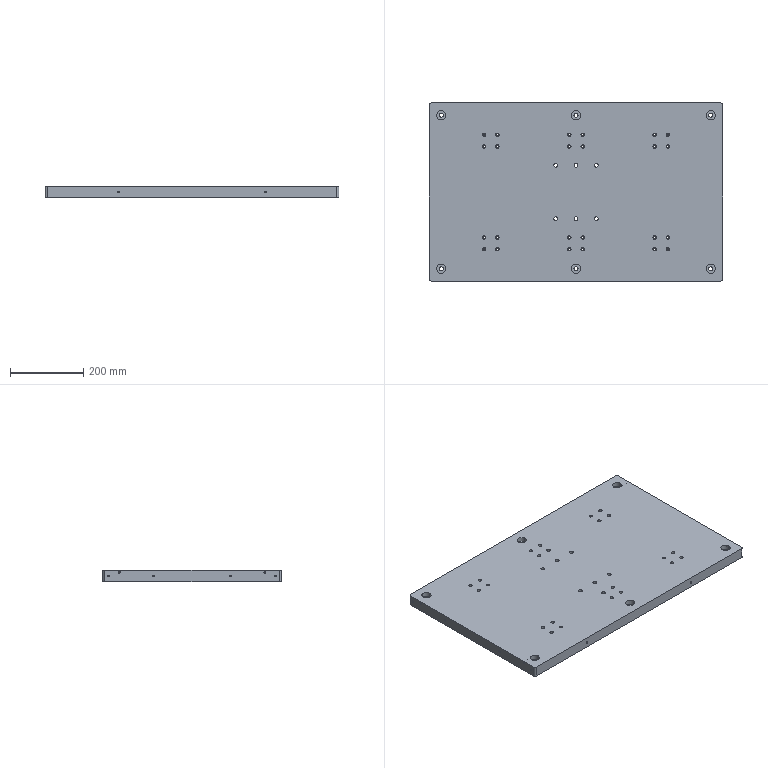NC program | Mastercam | posted with a generic post | part box 800 x 485 x 30 mm
Lines 4757 to 5950 of 7047:
N7890 T9 M6
N7900 G0 G90 G17 G54 X-361.57 Y208. A0. S6500 M3
N7910 G43 H9 Z50. M8
N7920 Z1.
N7930 G1 Z0. F600.
N7940 X-360.57 F3000.
N7950 G3 X-359.57 Y209. I0. J1.
N7960 X-367. Y216.43 Z-.175 I-7.43 J0.
N7970 X-374.43 Y209. Z-.35 I0. J-7.43
N7980 X-367. Y201.57 Z-.525 I7.43 J0.
N7990 X-359.57 Y209. Z-.7 I0. J7.43
N8000 X-367. Y216.43 Z-.875 I-7.43 J0.
N8010 X-374.43 Y209. Z-1.05 I0. J-7.43
N8020 X-367. Y201.57 Z-1.225 I7.43 J0.
N8030 X-359.57 Y209. Z-1.4 I0. J7.43
N8040 X-367. Y216.43 Z-1.575 I-7.43 J0.
N8050 X-374.43 Y209. Z-1.75 I0. J-7.43
N8060 X-367. Y201.57 Z-1.925 I7.43 J0.
N8070 X-359.57 Y209. Z-2.1 I0. J7.43
N8080 X-367. Y216.43 Z-2.275 I-7.43 J0.
N8090 X-374.43 Y209. Z-2.45 I0. J-7.43
N8100 X-367. Y201.57 Z-2.625 I7.43 J0.
N8110 X-359.57 Y209. Z-2.8 I0. J7.43
N8120 X-367. Y216.43 Z-2.975 I-7.43 J0.
N8130 X-374.43 Y209. Z-3.15 I0. J-7.43
N8140 X-367. Y201.57 Z-3.325 I7.43 J0.
N8150 X-359.57 Y209. Z-3.5 I0. J7.43
N8160 X-367. Y216.43 Z-3.675 I-7.43 J0.
N8170 X-374.43 Y209. Z-3.85 I0. J-7.43
N8180 X-367. Y201.57 Z-4.025 I7.43 J0.
N8190 X-359.57 Y209. Z-4.2 I0. J7.43
N8200 X-367. Y216.43 Z-4.375 I-7.43 J0.
N8210 X-374.43 Y209. Z-4.55 I0. J-7.43
N8220 X-367. Y201.57 Z-4.725 I7.43 J0.
N8230 X-359.57 Y209. Z-4.9 I0. J7.43
N8240 X-367. Y216.43 Z-5.075 I-7.43 J0.
N8250 X-374.43 Y209. Z-5.25 I0. J-7.43
N8260 X-367. Y201.57 Z-5.425 I7.43 J0.
N8270 X-359.57 Y209. Z-5.6 I0. J7.43
N8280 X-367. Y216.43 Z-5.775 I-7.43 J0.
N8290 X-374.43 Y209. Z-5.95 I0. J-7.43
N8300 X-367. Y201.57 Z-6.125 I7.43 J0.
N8310 X-359.57 Y209. Z-6.3 I0. J7.43
N8320 X-367. Y216.43 Z-6.475 I-7.43 J0.
N8330 X-374.43 Y209. Z-6.65 I0. J-7.43
N8340 X-367. Y201.57 Z-6.825 I7.43 J0.
N8350 X-359.57 Y209. Z-7. I0. J7.43
N8360 X-367. Y216.43 Z-7.175 I-7.43 J0.
N8370 X-374.43 Y209. Z-7.35 I0. J-7.43
N8380 X-367. Y201.57 Z-7.525 I7.43 J0.
N8390 X-359.57 Y209. Z-7.7 I0. J7.43
N8400 X-367. Y216.43 Z-7.875 I-7.43 J0.
N8410 X-374.43 Y209. Z-8.05 I0. J-7.43
N8420 X-367. Y201.57 Z-8.225 I7.43 J0.
N8430 X-359.57 Y209. Z-8.4 I0. J7.43
N8440 X-367. Y216.43 Z-8.575 I-7.43 J0.
N8450 X-374.43 Y209. Z-8.75 I0. J-7.43
N8460 X-367. Y201.57 Z-8.925 I7.43 J0.
N8470 X-359.57 Y209. Z-9.1 I0. J7.43
N8480 X-367. Y216.43 Z-9.275 I-7.43 J0.
N8490 X-374.43 Y209. Z-9.45 I0. J-7.43
N8500 X-367. Y201.57 Z-9.625 I7.43 J0.
N8510 X-359.57 Y209. Z-9.8 I0. J7.43
N8520 X-367. Y216.43 Z-9.975 I-7.43 J0.
N8530 X-374.43 Y209. Z-10.15 I0. J-7.43
N8540 X-367. Y201.57 Z-10.325 I7.43 J0.
N8550 X-359.57 Y209. Z-10.5 I0. J7.43
N8560 X-367. Y216.43 Z-10.675 I-7.43 J0.
N8570 X-374.43 Y209. Z-10.85 I0. J-7.43
N8580 X-367. Y201.57 Z-11.025 I7.43 J0.
N8590 X-359.57 Y209. Z-11.2 I0. J7.43
N8600 X-367. Y216.43 Z-11.375 I-7.43 J0.
N8610 X-374.43 Y209. Z-11.55 I0. J-7.43
N8620 X-367. Y201.57 Z-11.725 I7.43 J0.
N8630 X-359.57 Y209. Z-11.9 I0. J7.43
N8640 X-367. Y216.43 Z-12.075 I-7.43 J0.
N8650 X-374.43 Y209. Z-12.25 I0. J-7.43
N8660 X-367. Y201.57 Z-12.425 I7.43 J0.
N8670 X-359.57 Y209. Z-12.6 I0. J7.43
N8680 X-367. Y216.43 Z-12.775 I-7.43 J0.
N8690 X-373.694 Y212.224 Z-12.9 I0. J-7.43
N8700 X-374.43 Y209. I6.694 J-3.224
N8710 X-367. Y201.57 I7.43 J0.
N8720 X-359.57 Y209. I0. J7.43
N8730 X-367. Y216.43 I-7.43 J0.
N8740 X-373.694 Y212.224 I0. J-7.43
N8750 X-373.793 Y211.79 I.901 J-.434
N8760 X-373.227 Y210.889 I1. J0.
N8770 G1 X-372.326 Y210.455
N8780 G0 Z50.
N8790 X-361.57 Y-210.
N8800 Z1.
N8810 G1 Z0. F600.
N8820 X-360.57 F3000.
N8830 G3 X-359.57 Y-209. I0. J1.
N8840 X-367. Y-201.57 Z-.175 I-7.43 J0.
N8850 X-374.43 Y-209. Z-.35 I0. J-7.43
N8860 X-367. Y-216.43 Z-.525 I7.43 J0.
N8870 X-359.57 Y-209. Z-.7 I0. J7.43
N8880 X-367. Y-201.57 Z-.875 I-7.43 J0.
N8890 X-374.43 Y-209. Z-1.05 I0. J-7.43
N8900 X-367. Y-216.43 Z-1.225 I7.43 J0.
N8910 X-359.57 Y-209. Z-1.4 I0. J7.43
N8920 X-367. Y-201.57 Z-1.575 I-7.43 J0.
N8930 X-374.43 Y-209. Z-1.75 I0. J-7.43
N8940 X-367. Y-216.43 Z-1.925 I7.43 J0.
N8950 X-359.57 Y-209. Z-2.1 I0. J7.43
N8960 X-367. Y-201.57 Z-2.275 I-7.43 J0.
N8970 X-374.43 Y-209. Z-2.45 I0. J-7.43
N8980 X-367. Y-216.43 Z-2.625 I7.43 J0.
N8990 X-359.57 Y-209. Z-2.8 I0. J7.43
N9000 X-367. Y-201.57 Z-2.975 I-7.43 J0.
N9010 X-374.43 Y-209. Z-3.15 I0. J-7.43
N9020 X-367. Y-216.43 Z-3.325 I7.43 J0.
N9030 X-359.57 Y-209. Z-3.5 I0. J7.43
N9040 X-367. Y-201.57 Z-3.675 I-7.43 J0.
N9050 X-374.43 Y-209. Z-3.85 I0. J-7.43
N9060 X-367. Y-216.43 Z-4.025 I7.43 J0.
N9070 X-359.57 Y-209. Z-4.2 I0. J7.43
N9080 X-367. Y-201.57 Z-4.375 I-7.43 J0.
N9090 X-374.43 Y-209. Z-4.55 I0. J-7.43
N9100 X-367. Y-216.43 Z-4.725 I7.43 J0.
N9110 X-359.57 Y-209. Z-4.9 I0. J7.43
N9120 X-367. Y-201.57 Z-5.075 I-7.43 J0.
N9130 X-374.43 Y-209. Z-5.25 I0. J-7.43
N9140 X-367. Y-216.43 Z-5.425 I7.43 J0.
N9150 X-359.57 Y-209. Z-5.6 I0. J7.43
N9160 X-367. Y-201.57 Z-5.775 I-7.43 J0.
N9170 X-374.43 Y-209. Z-5.95 I0. J-7.43
N9180 X-367. Y-216.43 Z-6.125 I7.43 J0.
N9190 X-359.57 Y-209. Z-6.3 I0. J7.43
N9200 X-367. Y-201.57 Z-6.475 I-7.43 J0.
N9210 X-374.43 Y-209. Z-6.65 I0. J-7.43
N9220 X-367. Y-216.43 Z-6.825 I7.43 J0.
N9230 X-359.57 Y-209. Z-7. I0. J7.43
N9240 X-367. Y-201.57 Z-7.175 I-7.43 J0.
N9250 X-374.43 Y-209. Z-7.35 I0. J-7.43
N9260 X-367. Y-216.43 Z-7.525 I7.43 J0.
N9270 X-359.57 Y-209. Z-7.7 I0. J7.43
N9280 X-367. Y-201.57 Z-7.875 I-7.43 J0.
N9290 X-374.43 Y-209. Z-8.05 I0. J-7.43
N9300 X-367. Y-216.43 Z-8.225 I7.43 J0.
N9310 X-359.57 Y-209. Z-8.4 I0. J7.43
N9320 X-367. Y-201.57 Z-8.575 I-7.43 J0.
N9330 X-374.43 Y-209. Z-8.75 I0. J-7.43
N9340 X-367. Y-216.43 Z-8.925 I7.43 J0.
N9350 X-359.57 Y-209. Z-9.1 I0. J7.43
N9360 X-367. Y-201.57 Z-9.275 I-7.43 J0.
N9370 X-374.43 Y-209. Z-9.45 I0. J-7.43
N9380 X-367. Y-216.43 Z-9.625 I7.43 J0.
N9390 X-359.57 Y-209. Z-9.8 I0. J7.43
N9400 X-367. Y-201.57 Z-9.975 I-7.43 J0.
N9410 X-374.43 Y-209. Z-10.15 I0. J-7.43
N9420 X-367. Y-216.43 Z-10.325 I7.43 J0.
N9430 X-359.57 Y-209. Z-10.5 I0. J7.43
N9440 X-367. Y-201.57 Z-10.675 I-7.43 J0.
N9450 X-374.43 Y-209. Z-10.85 I0. J-7.43
N9460 X-367. Y-216.43 Z-11.025 I7.43 J0.
N9470 X-359.57 Y-209. Z-11.2 I0. J7.43
N9480 X-367. Y-201.57 Z-11.375 I-7.43 J0.
N9490 X-374.43 Y-209. Z-11.55 I0. J-7.43
N9500 X-367. Y-216.43 Z-11.725 I7.43 J0.
N9510 X-359.57 Y-209. Z-11.9 I0. J7.43
N9520 X-367. Y-201.57 Z-12.075 I-7.43 J0.
N9530 X-374.43 Y-209. Z-12.25 I0. J-7.43
N9540 X-367. Y-216.43 Z-12.425 I7.43 J0.
N9550 X-359.57 Y-209. Z-12.6 I0. J7.43
N9560 X-367. Y-201.57 Z-12.775 I-7.43 J0.
N9570 X-373.694 Y-205.776 Z-12.9 I0. J-7.43
N9580 X-374.43 Y-209. I6.694 J-3.224
N9590 X-367. Y-216.43 I7.43 J0.
N9600 X-359.57 Y-209. I0. J7.43
N9610 X-367. Y-201.57 I-7.43 J0.
N9620 X-373.694 Y-205.776 I0. J-7.43
N9630 X-373.793 Y-206.21 I.901 J-.434
N9640 X-373.227 Y-207.111 I1. J0.
N9650 G1 X-372.326 Y-207.545
N9660 G0 Z50.
N9670 X5.43 Y-210.
N9680 Z1.
N9690 G1 Z0. F600.
N9700 X6.43 F3000.
N9710 G3 X7.43 Y-209. I0. J1.
N9720 X0. Y-201.57 Z-.175 I-7.43 J0.
N9730 X-7.43 Y-209. Z-.35 I0. J-7.43
N9740 X0. Y-216.43 Z-.525 I7.43 J0.
N9750 X7.43 Y-209. Z-.7 I0. J7.43
N9760 X0. Y-201.57 Z-.875 I-7.43 J0.
N9770 X-7.43 Y-209. Z-1.05 I0. J-7.43
N9780 X0. Y-216.43 Z-1.225 I7.43 J0.
N9790 X7.43 Y-209. Z-1.4 I0. J7.43
N9800 X0. Y-201.57 Z-1.575 I-7.43 J0.
N9810 X-7.43 Y-209. Z-1.75 I0. J-7.43
N9820 X0. Y-216.43 Z-1.925 I7.43 J0.
N9830 X7.43 Y-209. Z-2.1 I0. J7.43
N9840 X0. Y-201.57 Z-2.275 I-7.43 J0.
N9850 X-7.43 Y-209. Z-2.45 I0. J-7.43
N9860 X0. Y-216.43 Z-2.625 I7.43 J0.
N9870 X7.43 Y-209. Z-2.8 I0. J7.43
N9880 X0. Y-201.57 Z-2.975 I-7.43 J0.
N9890 X-7.43 Y-209. Z-3.15 I0. J-7.43
N9900 X0. Y-216.43 Z-3.325 I7.43 J0.
N9910 X7.43 Y-209. Z-3.5 I0. J7.43
N9920 X0. Y-201.57 Z-3.675 I-7.43 J0.
N9930 X-7.43 Y-209. Z-3.85 I0. J-7.43
N9940 X0. Y-216.43 Z-4.025 I7.43 J0.
N9950 X7.43 Y-209. Z-4.2 I0. J7.43
N9960 X0. Y-201.57 Z-4.375 I-7.43 J0.
N9970 X-7.43 Y-209. Z-4.55 I0. J-7.43
N9980 X0. Y-216.43 Z-4.725 I7.43 J0.
N9990 X7.43 Y-209. Z-4.9 I0. J7.43
N100 X0. Y-201.57 Z-5.075 I-7.43 J0.
N110 X-7.43 Y-209. Z-5.25 I0. J-7.43
N120 X0. Y-216.43 Z-5.425 I7.43 J0.
N130 X7.43 Y-209. Z-5.6 I0. J7.43
N140 X0. Y-201.57 Z-5.775 I-7.43 J0.
N150 X-7.43 Y-209. Z-5.95 I0. J-7.43
N160 X0. Y-216.43 Z-6.125 I7.43 J0.
N170 X7.43 Y-209. Z-6.3 I0. J7.43
N180 X0. Y-201.57 Z-6.475 I-7.43 J0.
N190 X-7.43 Y-209. Z-6.65 I0. J-7.43
N200 X0. Y-216.43 Z-6.825 I7.43 J0.
N210 X7.43 Y-209. Z-7. I0. J7.43
N220 X0. Y-201.57 Z-7.175 I-7.43 J0.
N230 X-7.43 Y-209. Z-7.35 I0. J-7.43
N240 X0. Y-216.43 Z-7.525 I7.43 J0.
N250 X7.43 Y-209. Z-7.7 I0. J7.43
N260 X0. Y-201.57 Z-7.875 I-7.43 J0.
N270 X-7.43 Y-209. Z-8.05 I0. J-7.43
N280 X0. Y-216.43 Z-8.225 I7.43 J0.
N290 X7.43 Y-209. Z-8.4 I0. J7.43
N300 X0. Y-201.57 Z-8.575 I-7.43 J0.
N310 X-7.43 Y-209. Z-8.75 I0. J-7.43
N320 X0. Y-216.43 Z-8.925 I7.43 J0.
N330 X7.43 Y-209. Z-9.1 I0. J7.43
N340 X0. Y-201.57 Z-9.275 I-7.43 J0.
N350 X-7.43 Y-209. Z-9.45 I0. J-7.43
N360 X0. Y-216.43 Z-9.625 I7.43 J0.
N370 X7.43 Y-209. Z-9.8 I0. J7.43
N380 X0. Y-201.57 Z-9.975 I-7.43 J0.
N390 X-7.43 Y-209. Z-10.15 I0. J-7.43
N400 X0. Y-216.43 Z-10.325 I7.43 J0.
N410 X7.43 Y-209. Z-10.5 I0. J7.43
N420 X0. Y-201.57 Z-10.675 I-7.43 J0.
N430 X-7.43 Y-209. Z-10.85 I0. J-7.43
N440 X0. Y-216.43 Z-11.025 I7.43 J0.
N450 X7.43 Y-209. Z-11.2 I0. J7.43
N460 X0. Y-201.57 Z-11.375 I-7.43 J0.
N470 X-7.43 Y-209. Z-11.55 I0. J-7.43
N480 X0. Y-216.43 Z-11.725 I7.43 J0.
N490 X7.43 Y-209. Z-11.9 I0. J7.43
N500 X0. Y-201.57 Z-12.075 I-7.43 J0.
N510 X-7.43 Y-209. Z-12.25 I0. J-7.43
N520 X0. Y-216.43 Z-12.425 I7.43 J0.
N530 X7.43 Y-209. Z-12.6 I0. J7.43
N540 X0. Y-201.57 Z-12.775 I-7.43 J0.
N550 X-6.694 Y-205.776 Z-12.9 I0. J-7.43
N560 X-7.43 Y-209. I6.694 J-3.224
N570 X0. Y-216.43 I7.43 J0.
N580 X7.43 Y-209. I0. J7.43
N590 X0. Y-201.57 I-7.43 J0.
N600 X-6.694 Y-205.776 I0. J-7.43
N610 X-6.793 Y-206.21 I.901 J-.434
N620 X-6.227 Y-207.111 I1. J0.
N630 G1 X-5.326 Y-207.545
N640 G0 Z50.
N650 X5.43 Y208.
N660 Z1.
N670 G1 Z0. F600.
N680 X6.43 F3000.
N690 G3 X7.43 Y209. I0. J1.
N700 X0. Y216.43 Z-.175 I-7.43 J0.
N710 X-7.43 Y209. Z-.35 I0. J-7.43
N720 X0. Y201.57 Z-.525 I7.43 J0.
N730 X7.43 Y209. Z-.7 I0. J7.43
N740 X0. Y216.43 Z-.875 I-7.43 J0.
N750 X-7.43 Y209. Z-1.05 I0. J-7.43
N760 X0. Y201.57 Z-1.225 I7.43 J0.
N770 X7.43 Y209. Z-1.4 I0. J7.43
N780 X0. Y216.43 Z-1.575 I-7.43 J0.
N790 X-7.43 Y209. Z-1.75 I0. J-7.43
N800 X0. Y201.57 Z-1.925 I7.43 J0.
N810 X7.43 Y209. Z-2.1 I0. J7.43
N820 X0. Y216.43 Z-2.275 I-7.43 J0.
N830 X-7.43 Y209. Z-2.45 I0. J-7.43
N840 X0. Y201.57 Z-2.625 I7.43 J0.
N850 X7.43 Y209. Z-2.8 I0. J7.43
N860 X0. Y216.43 Z-2.975 I-7.43 J0.
N870 X-7.43 Y209. Z-3.15 I0. J-7.43
N880 X0. Y201.57 Z-3.325 I7.43 J0.
N890 X7.43 Y209. Z-3.5 I0. J7.43
N900 X0. Y216.43 Z-3.675 I-7.43 J0.
N910 X-7.43 Y209. Z-3.85 I0. J-7.43
N920 X0. Y201.57 Z-4.025 I7.43 J0.
N930 X7.43 Y209. Z-4.2 I0. J7.43
N940 X0. Y216.43 Z-4.375 I-7.43 J0.
N950 X-7.43 Y209. Z-4.55 I0. J-7.43
N960 X0. Y201.57 Z-4.725 I7.43 J0.
N970 X7.43 Y209. Z-4.9 I0. J7.43
N980 X0. Y216.43 Z-5.075 I-7.43 J0.
N990 X-7.43 Y209. Z-5.25 I0. J-7.43
N1000 X0. Y201.57 Z-5.425 I7.43 J0.
N1010 X7.43 Y209. Z-5.6 I0. J7.43
N1020 X0. Y216.43 Z-5.775 I-7.43 J0.
N1030 X-7.43 Y209. Z-5.95 I0. J-7.43
N1040 X0. Y201.57 Z-6.125 I7.43 J0.
N1050 X7.43 Y209. Z-6.3 I0. J7.43
N1060 X0. Y216.43 Z-6.475 I-7.43 J0.
N1070 X-7.43 Y209. Z-6.65 I0. J-7.43
N1080 X0. Y201.57 Z-6.825 I7.43 J0.
N1090 X7.43 Y209. Z-7. I0. J7.43
N1100 X0. Y216.43 Z-7.175 I-7.43 J0.
N1110 X-7.43 Y209. Z-7.35 I0. J-7.43
N1120 X0. Y201.57 Z-7.525 I7.43 J0.
N1130 X7.43 Y209. Z-7.7 I0. J7.43
N1140 X0. Y216.43 Z-7.875 I-7.43 J0.
N1150 X-7.43 Y209. Z-8.05 I0. J-7.43
N1160 X0. Y201.57 Z-8.225 I7.43 J0.
N1170 X7.43 Y209. Z-8.4 I0. J7.43
N1180 X0. Y216.43 Z-8.575 I-7.43 J0.
N1190 X-7.43 Y209. Z-8.75 I0. J-7.43
N1200 X0. Y201.57 Z-8.925 I7.43 J0.
N1210 X7.43 Y209. Z-9.1 I0. J7.43
N1220 X0. Y216.43 Z-9.275 I-7.43 J0.
N1230 X-7.43 Y209. Z-9.45 I0. J-7.43
N1240 X0. Y201.57 Z-9.625 I7.43 J0.
N1250 X7.43 Y209. Z-9.8 I0. J7.43
N1260 X0. Y216.43 Z-9.975 I-7.43 J0.
N1270 X-7.43 Y209. Z-10.15 I0. J-7.43
N1280 X0. Y201.57 Z-10.325 I7.43 J0.
N1290 X7.43 Y209. Z-10.5 I0. J7.43
N1300 X0. Y216.43 Z-10.675 I-7.43 J0.
N1310 X-7.43 Y209. Z-10.85 I0. J-7.43
N1320 X0. Y201.57 Z-11.025 I7.43 J0.
N1330 X7.43 Y209. Z-11.2 I0. J7.43
N1340 X0. Y216.43 Z-11.375 I-7.43 J0.
N1350 X-7.43 Y209. Z-11.55 I0. J-7.43
N1360 X0. Y201.57 Z-11.725 I7.43 J0.
N1370 X7.43 Y209. Z-11.9 I0. J7.43
N1380 X0. Y216.43 Z-12.075 I-7.43 J0.
N1390 X-7.43 Y209. Z-12.25 I0. J-7.43
N1400 X0. Y201.57 Z-12.425 I7.43 J0.
N1410 X7.43 Y209. Z-12.6 I0. J7.43
N1420 X0. Y216.43 Z-12.775 I-7.43 J0.
N1430 X-6.694 Y212.224 Z-12.9 I0. J-7.43
N1440 X-7.43 Y209. I6.694 J-3.224
N1450 X0. Y201.57 I7.43 J0.
N1460 X7.43 Y209. I0. J7.43
N1470 X0. Y216.43 I-7.43 J0.
N1480 X-6.694 Y212.224 I0. J-7.43
N1490 X-6.793 Y211.79 I.901 J-.434
N1500 X-6.227 Y210.889 I1. J0.
N1510 G1 X-5.326 Y210.455
N1520 G0 Z50.
N1530 X372.43 Y208.
N1540 Z1.
N1550 G1 Z0. F600.
N1560 X373.43 F3000.
N1570 G3 X374.43 Y209. I0. J1.
N1580 X367. Y216.43 Z-.175 I-7.43 J0.
N1590 X359.57 Y209. Z-.35 I0. J-7.43
N1600 X367. Y201.57 Z-.525 I7.43 J0.
N1610 X374.43 Y209. Z-.7 I0. J7.43
N1620 X367. Y216.43 Z-.875 I-7.43 J0.
N1630 X359.57 Y209. Z-1.05 I0. J-7.43
N1640 X367. Y201.57 Z-1.225 I7.43 J0.
N1650 X374.43 Y209. Z-1.4 I0. J7.43
N1660 X367. Y216.43 Z-1.575 I-7.43 J0.
N1670 X359.57 Y209. Z-1.75 I0. J-7.43
N1680 X367. Y201.57 Z-1.925 I7.43 J0.
N1690 X374.43 Y209. Z-2.1 I0. J7.43
N1700 X367. Y216.43 Z-2.275 I-7.43 J0.
N1710 X359.57 Y209. Z-2.45 I0. J-7.43
N1720 X367. Y201.57 Z-2.625 I7.43 J0.
N1730 X374.43 Y209. Z-2.8 I0. J7.43
N1740 X367. Y216.43 Z-2.975 I-7.43 J0.
N1750 X359.57 Y209. Z-3.15 I0. J-7.43
N1760 X367. Y201.57 Z-3.325 I7.43 J0.
N1770 X374.43 Y209. Z-3.5 I0. J7.43
N1780 X367. Y216.43 Z-3.675 I-7.43 J0.
N1790 X359.57 Y209. Z-3.85 I0. J-7.43
N1800 X367. Y201.57 Z-4.025 I7.43 J0.
N1810 X374.43 Y209. Z-4.2 I0. J7.43
N1820 X367. Y216.43 Z-4.375 I-7.43 J0.
N1830 X359.57 Y209. Z-4.55 I0. J-7.43
N1840 X367. Y201.57 Z-4.725 I7.43 J0.
N1850 X374.43 Y209. Z-4.9 I0. J7.43
N1860 X367. Y216.43 Z-5.075 I-7.43 J0.
N1870 X359.57 Y209. Z-5.25 I0. J-7.43
N1880 X367. Y201.57 Z-5.425 I7.43 J0.
N1890 X374.43 Y209. Z-5.6 I0. J7.43
N1900 X367. Y216.43 Z-5.775 I-7.43 J0.
N1910 X359.57 Y209. Z-5.95 I0. J-7.43
N1920 X367. Y201.57 Z-6.125 I7.43 J0.
N1930 X374.43 Y209. Z-6.3 I0. J7.43
N1940 X367. Y216.43 Z-6.475 I-7.43 J0.
N1950 X359.57 Y209. Z-6.65 I0. J-7.43
N1960 X367. Y201.57 Z-6.825 I7.43 J0.
N1970 X374.43 Y209. Z-7. I0. J7.43
N1980 X367. Y216.43 Z-7.175 I-7.43 J0.
N1990 X359.57 Y209. Z-7.35 I0. J-7.43
N2000 X367. Y201.57 Z-7.525 I7.43 J0.
N2010 X374.43 Y209. Z-7.7 I0. J7.43
N2020 X367. Y216.43 Z-7.875 I-7.43 J0.
N2030 X359.57 Y209. Z-8.05 I0. J-7.43
N2040 X367. Y201.57 Z-8.225 I7.43 J0.
N2050 X374.43 Y209. Z-8.4 I0. J7.43
N2060 X367. Y216.43 Z-8.575 I-7.43 J0.
N2070 X359.57 Y209. Z-8.75 I0. J-7.43
N2080 X367. Y201.57 Z-8.925 I7.43 J0.
N2090 X374.43 Y209. Z-9.1 I0. J7.43
N2100 X367. Y216.43 Z-9.275 I-7.43 J0.
N2110 X359.57 Y209. Z-9.45 I0. J-7.43
N2120 X367. Y201.57 Z-9.625 I7.43 J0.
N2130 X374.43 Y209. Z-9.8 I0. J7.43
N2140 X367. Y216.43 Z-9.975 I-7.43 J0.
N2150 X359.57 Y209. Z-10.15 I0. J-7.43
N2160 X367. Y201.57 Z-10.325 I7.43 J0.
N2170 X374.43 Y209. Z-10.5 I0. J7.43
N2180 X367. Y216.43 Z-10.675 I-7.43 J0.
N2190 X359.57 Y209. Z-10.85 I0. J-7.43
N2200 X367. Y201.57 Z-11.025 I7.43 J0.
N2210 X374.43 Y209. Z-11.2 I0. J7.43
N2220 X367. Y216.43 Z-11.375 I-7.43 J0.
N2230 X359.57 Y209. Z-11.55 I0. J-7.43
N2240 X367. Y201.57 Z-11.725 I7.43 J0.
N2250 X374.43 Y209. Z-11.9 I0. J7.43
N2260 X367. Y216.43 Z-12.075 I-7.43 J0.
N2270 X359.57 Y209. Z-12.25 I0. J-7.43
N2280 X367. Y201.57 Z-12.425 I7.43 J0.
N2290 X374.43 Y209. Z-12.6 I0. J7.43
N2300 X367. Y216.43 Z-12.775 I-7.43 J0.
N2310 X360.306 Y212.224 Z-12.9 I0. J-7.43
N2320 X359.57 Y209. I6.694 J-3.224
N2330 X367. Y201.57 I7.43 J0.
N2340 X374.43 Y209. I0. J7.43
N2350 X367. Y216.43 I-7.43 J0.
N2360 X360.306 Y212.224 I0. J-7.43
N2370 X360.207 Y211.79 I.901 J-.434
N2380 X360.773 Y210.889 I1. J0.
N2390 G1 X361.674 Y210.455
N2400 G0 Z50.
N2410 X372.43 Y-210.
N2420 Z1.
N2430 G1 Z0. F600.
N2440 X373.43 F3000.
N2450 G3 X374.43 Y-209. I0. J1.
N2460 X367. Y-201.57 Z-.175 I-7.43 J0.
N2470 X359.57 Y-209. Z-.35 I0. J-7.43
N2480 X367. Y-216.43 Z-.525 I7.43 J0.
N2490 X374.43 Y-209. Z-.7 I0. J7.43
N2500 X367. Y-201.57 Z-.875 I-7.43 J0.
N2510 X359.57 Y-209. Z-1.05 I0. J-7.43
N2520 X367. Y-216.43 Z-1.225 I7.43 J0.
N2530 X374.43 Y-209. Z-1.4 I0. J7.43
N2540 X367. Y-201.57 Z-1.575 I-7.43 J0.
N2550 X359.57 Y-209. Z-1.75 I0. J-7.43
N2560 X367. Y-216.43 Z-1.925 I7.43 J0.
N2570 X374.43 Y-209. Z-2.1 I0. J7.43
N2580 X367. Y-201.57 Z-2.275 I-7.43 J0.
N2590 X359.57 Y-209. Z-2.45 I0. J-7.43
N2600 X367. Y-216.43 Z-2.625 I7.43 J0.
N2610 X374.43 Y-209. Z-2.8 I0. J7.43
N2620 X367. Y-201.57 Z-2.975 I-7.43 J0.
N2630 X359.57 Y-209. Z-3.15 I0. J-7.43
N2640 X367. Y-216.43 Z-3.325 I7.43 J0.
N2650 X374.43 Y-209. Z-3.5 I0. J7.43
N2660 X367. Y-201.57 Z-3.675 I-7.43 J0.
N2670 X359.57 Y-209. Z-3.85 I0. J-7.43
N2680 X367. Y-216.43 Z-4.025 I7.43 J0.
N2690 X374.43 Y-209. Z-4.2 I0. J7.43
N2700 X367. Y-201.57 Z-4.375 I-7.43 J0.
N2710 X359.57 Y-209. Z-4.55 I0. J-7.43
N2720 X367. Y-216.43 Z-4.725 I7.43 J0.
N2730 X374.43 Y-209. Z-4.9 I0. J7.43
N2740 X367. Y-201.57 Z-5.075 I-7.43 J0.
N2750 X359.57 Y-209. Z-5.25 I0. J-7.43
N2760 X367. Y-216.43 Z-5.425 I7.43 J0.
N2770 X374.43 Y-209. Z-5.6 I0. J7.43
N2780 X367. Y-201.57 Z-5.775 I-7.43 J0.
N2790 X359.57 Y-209. Z-5.95 I0. J-7.43
N2800 X367. Y-216.43 Z-6.125 I7.43 J0.
N2810 X374.43 Y-209. Z-6.3 I0. J7.43
N2820 X367. Y-201.57 Z-6.475 I-7.43 J0.
N2830 X359.57 Y-209. Z-6.65 I0. J-7.43
N2840 X367. Y-216.43 Z-6.825 I7.43 J0.
N2850 X374.43 Y-209. Z-7. I0. J7.43
N2860 X367. Y-201.57 Z-7.175 I-7.43 J0.
N2870 X359.57 Y-209. Z-7.35 I0. J-7.43
N2880 X367. Y-216.43 Z-7.525 I7.43 J0.
N2890 X374.43 Y-209. Z-7.7 I0. J7.43
N2900 X367. Y-201.57 Z-7.875 I-7.43 J0.
N2910 X359.57 Y-209. Z-8.05 I0. J-7.43
N2920 X367. Y-216.43 Z-8.225 I7.43 J0.
N2930 X374.43 Y-209. Z-8.4 I0. J7.43
N2940 X367. Y-201.57 Z-8.575 I-7.43 J0.
N2950 X359.57 Y-209. Z-8.75 I0. J-7.43
N2960 X367. Y-216.43 Z-8.925 I7.43 J0.
N2970 X374.43 Y-209. Z-9.1 I0. J7.43
N2980 X367. Y-201.57 Z-9.275 I-7.43 J0.
N2990 X359.57 Y-209. Z-9.45 I0. J-7.43
N3000 X367. Y-216.43 Z-9.625 I7.43 J0.
N3010 X374.43 Y-209. Z-9.8 I0. J7.43
N3020 X367. Y-201.57 Z-9.975 I-7.43 J0.
N3030 X359.57 Y-209. Z-10.15 I0. J-7.43
N3040 X367. Y-216.43 Z-10.325 I7.43 J0.
N3050 X374.43 Y-209. Z-10.5 I0. J7.43
N3060 X367. Y-201.57 Z-10.675 I-7.43 J0.
N3070 X359.57 Y-209. Z-10.85 I0. J-7.43
N3080 X367. Y-216.43 Z-11.025 I7.43 J0.
N3090 X374.43 Y-209. Z-11.2 I0. J7.43
N3100 X367. Y-201.57 Z-11.375 I-7.43 J0.
N3110 X359.57 Y-209. Z-11.55 I0. J-7.43
N3120 X367. Y-216.43 Z-11.725 I7.43 J0.
N3130 X374.43 Y-209. Z-11.9 I0. J7.43
N3140 X367. Y-201.57 Z-12.075 I-7.43 J0.
N3150 X359.57 Y-209. Z-12.25 I0. J-7.43
N3160 X367. Y-216.43 Z-12.425 I7.43 J0.
N3170 X374.43 Y-209. Z-12.6 I0. J7.43
N3180 X367. Y-201.57 Z-12.775 I-7.43 J0.
N3190 X360.306 Y-205.776 Z-12.9 I0. J-7.43
N3200 X359.57 Y-209. I6.694 J-3.224
N3210 X367. Y-216.43 I7.43 J0.
N3220 X374.43 Y-209. I0. J7.43
N3230 X367. Y-201.57 I-7.43 J0.
N3240 X360.306 Y-205.776 I0. J-7.43
N3250 X360.207 Y-206.21 I.901 J-.434
N3260 X360.773 Y-207.111 I1. J0.
N3270 G1 X361.674 Y-207.545
N3280 G0 Z50.
N3290 M5
N3300 G91 G28 Z0. M9
N3310 A0.
N3320 M01
N3330 T10 M6
N3340 G0 G90 G17 G54 X-361.48 Y208. A0. S6500 M3
N3350 G43 H10 Z50. M8
N3360 Z1.
N3370 G1 Z-13. F600.
N3380 G41 D10 X-360.48 F1000.
N3390 G3 X-359.48 Y209. I0. J1.
N3400 X-367. Y216.52 I-7.52 J0.
N3410 X-374.52 Y209. I0. J-7.52
N3420 X-367. Y201.48 I7.52 J0.
N3430 X-359.48 Y209. I0. J7.52
N3440 X-360.48 Y210. I-1. J0.
N3450 G1 G40 X-361.48
N3460 G0 Z50.
N3470 Y208.
N3480 Z1.
N3490 G1 Z-13. F600.
N3500 G41 D10 X-360.48 F1000.
N3510 G3 X-359.48 Y209. I0. J1.
N3520 X-367. Y216.52 I-7.52 J0.
N3530 X-374.52 Y209. I0. J-7.52
N3540 X-367. Y201.48 I7.52 J0.
N3550 X-359.48 Y209. I0. J7.52
N3560 X-360.48 Y210. I-1. J0.
N3570 G1 G40 X-361.48
N3580 G0 Z50.
N3590 Y-210.
N3600 Z1.
N3610 G1 Z-13. F600.
N3620 G41 D10 X-360.48 F1000.
N3630 G3 X-359.48 Y-209. I0. J1.
N3640 X-367. Y-201.48 I-7.52 J0.
N3650 X-374.52 Y-209. I0. J-7.52
N3660 X-367. Y-216.52 I7.52 J0.
N3670 X-359.48 Y-209. I0. J7.52
N3680 X-360.48 Y-208. I-1. J0.
N3690 G1 G40 X-361.48
N3700 G0 Z50.
N3710 Y-210.
N3720 Z1.
N3730 G1 Z-13. F600.
N3740 G41 D10 X-360.48 F1000.
N3750 G3 X-359.48 Y-209. I0. J1.
N3760 X-367. Y-201.48 I-7.52 J0.
N3770 X-374.52 Y-209. I0. J-7.52
N3780 X-367. Y-216.52 I7.52 J0.
N3790 X-359.48 Y-209. I0. J7.52
N3800 X-360.48 Y-208. I-1. J0.
N3810 G1 G40 X-361.48
N3820 G0 Z50.
N3830 X5.52 Y-210.
N3840 Z1.
N3850 G1 Z-13. F600.
N3860 G41 D10 X6.52 F1000.
N3870 G3 X7.52 Y-209. I0. J1.
N3880 X0. Y-201.48 I-7.52 J0.
N3890 X-7.52 Y-209. I0. J-7.52
N3900 X0. Y-216.52 I7.52 J0.
N3910 X7.52 Y-209. I0. J7.52
N3920 X6.52 Y-208. I-1. J0.
N3930 G1 G40 X5.52
N3940 G0 Z50.
N3950 Y-210.
N3960 Z1.
N3970 G1 Z-13. F600.
N3980 G41 D10 X6.52 F1000.
N3990 G3 X7.52 Y-209. I0. J1.
N4000 X0. Y-201.48 I-7.52 J0.
N4010 X-7.52 Y-209. I0. J-7.52
N4020 X0. Y-216.52 I7.52 J0.
N4030 X7.52 Y-209. I0. J7.52
N4040 X6.52 Y-208. I-1. J0.
N4050 G1 G40 X5.52
N4060 G0 Z50.
N4070 Y208.
N4080 Z1.
N4090 G1 Z-13. F600.
N4100 G41 D10 X6.52 F1000.
N4110 G3 X7.52 Y209. I0. J1.
N4120 X0. Y216.52 I-7.52 J0.
N4130 X-7.52 Y209. I0. J-7.52
N4140 X0. Y201.48 I7.52 J0.
N4150 X7.52 Y209. I0. J7.52
N4160 X6.52 Y210. I-1. J0.
N4170 G1 G40 X5.52
N4180 G0 Z50.
N4190 Y208.
N4200 Z1.
N4210 G1 Z-13. F600.
N4220 G41 D10 X6.52 F1000.
N4230 G3 X7.52 Y209. I0. J1.
N4240 X0. Y216.52 I-7.52 J0.
N4250 X-7.52 Y209. I0. J-7.52
N4260 X0. Y201.48 I7.52 J0.
N4270 X7.52 Y209. I0. J7.52
N4280 X6.52 Y210. I-1. J0.
N4290 G1 G40 X5.52
N4300 G0 Z50.
N4310 X372.52 Y208.
N4320 Z1.
N4330 G1 Z-13. F600.
N4340 G41 D10 X373.52 F1000.
N4350 G3 X374.52 Y209. I0. J1.
N4360 X367. Y216.52 I-7.52 J0.
N4370 X359.48 Y209. I0. J-7.52
N4380 X367. Y201.48 I7.52 J0.
N4390 X374.52 Y209. I0. J7.52
N4400 X373.52 Y210. I-1. J0.
N4410 G1 G40 X372.52
N4420 G0 Z50.
N4430 Y208.
N4440 Z1.
N4450 G1 Z-13. F600.
N4460 G41 D10 X373.52 F1000.
N4470 G3 X374.52 Y209. I0. J1.
N4480 X367. Y216.52 I-7.52 J0.
N4490 X359.48 Y209. I0. J-7.52
N4500 X367. Y201.48 I7.52 J0.
N4510 X374.52 Y209. I0. J7.52
N4520 X373.52 Y210. I-1. J0.
N4530 G1 G40 X372.52
N4540 G0 Z50.
N4550 Y-210.
N4560 Z1.
N4570 G1 Z-13. F600.
N4580 G41 D10 X373.52 F1000.
N4590 G3 X374.52 Y-209. I0. J1.
N4600 X367. Y-201.48 I-7.52 J0.
N4610 X359.48 Y-209. I0. J-7.52
N4620 X367. Y-216.52 I7.52 J0.
N4630 X374.52 Y-209. I0. J7.52
N4640 X373.52 Y-208. I-1. J0.
N4650 G1 G40 X372.52
N4660 G0 Z50.
N4670 Y-210.
N4680 Z1.
N4690 G1 Z-13. F600.
N4700 G41 D10 X373.52 F1000.
N4710 G3 X374.52 Y-209. I0. J1.
N4720 X367. Y-201.48 I-7.52 J0.
N4730 X359.48 Y-209. I0. J-7.52
N4740 X367. Y-216.52 I7.52 J0.
N4750 X374.52 Y-209. I0. J7.52
N4760 X373.52 Y-208. I-1. J0.
N4770 G1 G40 X372.52
N4780 G0 Z50.
N4790 M5
N4800 G91 G28 Z0. M9
N4810 A0.
N4820 M01
N4830 T7 M6
N4840 G0 G90 G17 G54 X-51.2 Y-72.9 A0. S6000 M3
N4850 G43 H7 Z50. M8
N4860 Z1.
N4870 G1 Z-.8 F600.
N4880 X-50.8 F1000.
N4890 G3 X-50.4 Y-72.5 I0. J.4
N4900 X-55. Y-67.9 I-4.6 J0.
N4910 X-59.6 Y-72.5 I0. J-4.6
N4920 X-55. Y-77.1 I4.6 J0.
N4930 X-50.4 Y-72.5 I0. J4.6
N4940 X-50.8 Y-72.1 I-.4 J0.
N4950 G1 X-51.2
N4960 G0 Z50.
N4970 X3.8 Y-72.9
N4980 Z1.
N4990 G1 Z-.8 F600.
N5000 X4.2 F1000.
N5010 G3 X4.6 Y-72.5 I0. J.4
N5020 X0. Y-67.9 I-4.6 J0.
N5030 X-4.6 Y-72.5 I0. J-4.6
N5040 X0. Y-77.1 I4.6 J0.
N5050 X4.6 Y-72.5 I0. J4.6
N5060 X4.2 Y-72.1 I-.4 J0.
N5070 G1 X3.8
N5080 G0 Z50.
N5090 X58.8 Y-72.9
N5100 Z1.
N5110 G1 Z-.8 F600.
N5120 X59.2 F1000.
N5130 G3 X59.6 Y-72.5 I0. J.4
N5140 X55. Y-67.9 I-4.6 J0.
N5150 X50.4 Y-72.5 I0. J-4.6
N5160 X55. Y-77.1 I4.6 J0.
N5170 X59.6 Y-72.5 I0. J4.6
N5180 X59.2 Y-72.1 I-.4 J0.
N5190 G1 X58.8
N5200 G0 Z50.
N5210 X-51.2 Y72.1
N5220 Z1.
N5230 G1 Z-.8 F600.
N5240 X-50.8 F1000.
N5250 G3 X-50.4 Y72.5 I0. J.4
N5260 X-55. Y77.1 I-4.6 J0.
N5270 X-59.6 Y72.5 I0. J-4.6
N5280 X-55. Y67.9 I4.6 J0.
N5290 X-50.4 Y72.5 I0. J4.6
N5300 X-50.8 Y72.9 I-.4 J0.
N5310 G1 X-51.2
N5320 G0 Z50.
N5330 X3.8 Y72.1
N5340 Z1.
N5350 G1 Z-.8 F600.
N5360 X4.2 F1000.
N5370 G3 X4.6 Y72.5 I0. J.4
N5380 X0. Y77.1 I-4.6 J0.
N5390 X-4.6 Y72.5 I0. J-4.6
N5400 X0. Y67.9 I4.6 J0.
N5410 X4.6 Y72.5 I0. J4.6
N5420 X4.2 Y72.9 I-.4 J0.
N5430 G1 X3.8
N5440 G0 Z50.
N5450 X58.8 Y72.1
N5460 Z1.
N5470 G1 Z-.8 F600.
N5480 X59.2 F1000.
N5490 G3 X59.6 Y72.5 I0. J.4
N5500 X55. Y77.1 I-4.6 J0.
N5510 X50.4 Y72.5 I0. J-4.6
N5520 X55. Y67.9 I4.6 J0.
N5530 X59.6 Y72.5 I0. J4.6
N5540 X59.2 Y72.9 I-.4 J0.
N5550 G1 X58.8
N5560 G0 Z50.
N5570 X217.05 Y-124.4
N5580 Z1.
N5590 G1 Z-.8 F600.
N5600 X217.45 F1000.
N5610 G3 X217.85 Y-124. I0. J.4
N5620 X214. Y-120.15 I-3.85 J0.
N5630 X210.15 Y-124. I0. J-3.85
N5640 X214. Y-127.85 I3.85 J0.
N5650 X217.85 Y-124. I0. J3.85
N5660 X217.45 Y-123.6 I-.4 J0.
N5670 G1 X217.05
N5680 G0 Z50.
N5690 X253.05 Y155.6
N5700 Z1.
N5710 G1 Z-.8 F600.
N5720 X253.45 F1000.
N5730 G3 X253.85 Y156. I0. J.4
N5740 X250. Y159.85 I-3.85 J0.
N5750 X246.15 Y156. I0. J-3.85
N5760 X250. Y152.15 I3.85 J0.
N5770 X253.85 Y156. I0. J3.85
N5780 X253.45 Y156.4 I-.4 J0.
N5790 G1 X253.05
N5800 G0 Z50.
N5810 Y123.6
N5820 Z1.
N5830 G1 Z-.8 F600.
N5840 X253.45 F1000.
N5850 G3 X253.85 Y124. I0. J.4
N5860 X250. Y127.85 I-3.85 J0.
N5870 X246.15 Y124. I0. J-3.85
N5880 X250. Y120.15 I3.85 J0.
N5890 X253.85 Y124. I0. J3.85
N5900 X253.45 Y124.4 I-.4 J0.
N5910 G1 X253.05
N5920 G0 Z50.
N5930 X217.05 Y123.6
N5940 Z1.
N5950 G1 Z-.8 F600.
N5960 X217.45 F1000.
N5970 G3 X217.85 Y124. I0. J.4
N5980 X214. Y127.85 I-3.85 J0.
N5990 X210.15 Y124. I0. J-3.85
N6000 X214. Y120.15 I3.85 J0.
N6010 X217.85 Y124. I0. J3.85
N6020 X217.45 Y124.4 I-.4 J0.
N6030 G1 X217.05
N6040 G0 Z50.
N6050 Y-156.4
N6060 Z1.
N6070 G1 Z-.8 F600.
N6080 X217.45 F1000.
N6090 G3 X217.85 Y-156. I0. J.4
N6100 X214. Y-152.15 I-3.85 J0.
N6110 X210.15 Y-156. I0. J-3.85
N6120 X214. Y-159.85 I3.85 J0.
N6130 X217.85 Y-156. I0. J3.85
N6140 X217.45 Y-155.6 I-.4 J0.
N6150 G1 X217.05
N6160 G0 Z50.
N6170 X253.05 Y-156.4
N6180 Z1.
N6190 G1 Z-.8 F600.
N6200 X253.45 F1000.
N6210 G3 X253.85 Y-156. I0. J.4
N6220 X250. Y-152.15 I-3.85 J0.
N6230 X246.15 Y-156. I0. J-3.85
N6240 X250. Y-159.85 I3.85 J0.
N6250 X253.85 Y-156. I0. J3.85
N6260 X253.45 Y-155.6 I-.4 J0.
N6270 G1 X253.05
N6280 G0 Z50.
N6290 Y-124.4
N6300 Z1.
N6310 G1 Z-.8 F600.
N6320 X253.45 F1000.
N6330 G3 X253.85 Y-124. I0. J.4
N6340 X250. Y-120.15 I-3.85 J0.
N6350 X246.15 Y-124. I0. J-3.85
N6360 X250. Y-127.85 I3.85 J0.
N6370 X253.85 Y-124. I0. J3.85
N6380 X253.45 Y-123.6 I-.4 J0.
N6390 G1 X253.05
N6400 G0 Z50.
N6410 X21.05 Y-124.4
N6420 Z1.
N6430 G1 Z-.8 F600.
N6440 X21.45 F1000.
N6450 G3 X21.85 Y-124. I0. J.4
N6460 X18. Y-120.15 I-3.85 J0.
N6470 X14.15 Y-124. I0. J-3.85
N6480 X18. Y-127.85 I3.85 J0.
N6490 X21.85 Y-124. I0. J3.85
N6500 X21.45 Y-123.6 I-.4 J0.
N6510 G1 X21.05
N6520 G0 Z50.
N6530 X-246.95 Y123.6
N6540 Z1.
N6550 G1 Z-.8 F600.
N6560 X-246.55 F1000.
N6570 G3 X-246.15 Y124. I0. J.4
N6580 X-250. Y127.85 I-3.85 J0.
N6590 X-253.85 Y124. I0. J-3.85
N6600 X-250. Y120.15 I3.85 J0.
N6610 X-246.15 Y124. I0. J3.85
N6620 X-246.55 Y124.4 I-.4 J0.
N6630 G1 X-246.95
N6640 G0 Z50.
N6650 X-210.95 Y123.6
N6660 Z1.
N6670 G1 Z-.8 F600.
N6680 X-210.55 F1000.
N6690 G3 X-210.15 Y124. I0. J.4
N6700 X-214. Y127.85 I-3.85 J0.
N6710 X-217.85 Y124. I0. J-3.85
N6720 X-214. Y120.15 I3.85 J0.
N6730 X-210.15 Y124. I0. J3.85
N6740 X-210.55 Y124.4 I-.4 J0.
N6750 G1 X-210.95
N6760 G0 Z50.
N6770 Y155.6
N6780 Z1.
N6790 G1 Z-.8 F600.
N6800 X-210.55 F1000.
N6810 G3 X-210.15 Y156. I0. J.4
N6820 X-214. Y159.85 I-3.85 J0.
N6830 X-217.85 Y156. I0. J-3.85
N6840 X-214. Y152.15 I3.85 J0.
N6850 X-210.15 Y156. I0. J3.85
N6860 X-210.55 Y156.4 I-.4 J0.
N6870 G1 X-210.95
N6880 G0 Z50.
N6890 X-14.95 Y155.6
N6900 Z1.
N6910 G1 Z-.8 F600.
N6920 X-14.55 F1000.
N6930 G3 X-14.15 Y156. I0. J.4
N6940 X-18. Y159.85 I-3.85 J0.
N6950 X-21.85 Y156. I0. J-3.85
N6960 X-18. Y152.15 I3.85 J0.
N6970 X-14.15 Y156. I0. J3.85
N6980 X-14.55 Y156.4 I-.4 J0.
N6990 G1 X-14.95
N7000 G0 Z50.
N7010 Y123.6
N7020 Z1.
N7030 G1 Z-.8 F600.
N7040 X-14.55 F1000.
N7050 G3 X-14.15 Y124. I0. J.4
N7060 X-18. Y127.85 I-3.85 J0.
N7070 X-21.85 Y124. I0. J-3.85
N7080 X-18. Y120.15 I3.85 J0.
N7090 X-14.15 Y124. I0. J3.85
N7100 X-14.55 Y124.4 I-.4 J0.
N7110 G1 X-14.95
N7120 G0 Z50.
N7130 X21.05 Y123.6
N7140 Z1.
N7150 G1 Z-.8 F600.
N7160 X21.45 F1000.
N7170 G3 X21.85 Y124. I0. J.4
N7180 X18. Y127.85 I-3.85 J0.
N7190 X14.15 Y124. I0. J-3.85
N7200 X18. Y120.15 I3.85 J0.
N7210 X21.85 Y124. I0. J3.85
N7220 X21.45 Y124.4 I-.4 J0.
N7230 G1 X21.05
N7240 G0 Z50.
N7250 Y155.6
N7260 Z1.
N7270 G1 Z-.8 F600.
N7280 X21.45 F1000.
N7290 G3 X21.85 Y156. I0. J.4
N7300 X18. Y159.85 I-3.85 J0.
N7310 X14.15 Y156. I0. J-3.85
N7320 X18. Y152.15 I3.85 J0.
N7330 X21.85 Y156. I0. J3.85
N7340 X21.45 Y156.4 I-.4 J0.
N7350 G1 X21.05
N7360 G0 Z50.
N7370 X217.05 Y155.6
N7380 Z1.
N7390 G1 Z-.8 F600.
N7400 X217.45 F1000.
N7410 G3 X217.85 Y156. I0. J.4
N7420 X214. Y159.85 I-3.85 J0.
N7430 X210.15 Y156. I0. J-3.85
N7440 X214. Y152.15 I3.85 J0.
N7450 X217.85 Y156. I0. J3.85
N7460 X217.45 Y156.4 I-.4 J0.
N7470 G1 X217.05
N7480 G0 Z50.
N7490 X-210.95 Y-124.4
N7500 Z1.
N7510 G1 Z-.8 F600.
N7520 X-210.55 F1000.
N7530 G3 X-210.15 Y-124. I0. J.4
N7540 X-214. Y-120.15 I-3.85 J0.
N7550 X-217.85 Y-124. I0. J-3.85
N7560 X-214. Y-127.85 I3.85 J0.
N7570 X-210.15 Y-124. I0. J3.85
N7580 X-210.55 Y-123.6 I-.4 J0.
N7590 G1 X-210.95
N7600 G0 Z50.
N7610 Y-156.4
N7620 Z1.
N7630 G1 Z-.8 F600.
N7640 X-210.55 F1000.
N7650 G3 X-210.15 Y-156. I0. J.4
N7660 X-214. Y-152.15 I-3.85 J0.
N7670 X-217.85 Y-156. I0. J-3.85
N7680 X-214. Y-159.85 I3.85 J0.
N7690 X-210.15 Y-156. I0. J3.85
N7700 X-210.55 Y-155.6 I-.4 J0.
N7710 G1 X-210.95
N7720 G0 Z50.
N7730 X-246.95 Y-156.4
N7740 Z1.
N7750 G1 Z-.8 F600.
N7760 X-246.55 F1000.
N7770 G3 X-246.15 Y-156. I0. J.4
N7780 X-250. Y-152.15 I-3.85 J0.
N7790 X-253.85 Y-156. I0. J-3.85
N7800 X-250. Y-159.85 I3.85 J0.
N7810 X-246.15 Y-156. I0. J3.85
N7820 X-246.55 Y-155.6 I-.4 J0.
N7830 G1 X-246.95
N7840 G0 Z50.
N7850 Y-124.4
N7860 Z1.
N7870 G1 Z-.8 F600.
N7880 X-246.55 F1000.
N7890 G3 X-246.15 Y-124. I0. J.4
N7900 X-250. Y-120.15 I-3.85 J0.
N7910 X-253.85 Y-124. I0. J-3.85
N7920 X-250. Y-127.85 I3.85 J0.
N7930 X-246.15 Y-124. I0. J3.85
N7940 X-246.55 Y-123.6 I-.4 J0.
N7950 G1 X-246.95
N7960 G0 Z50.
N7970 X-14.95 Y-124.4
N7980 Z1.
N7990 G1 Z-.8 F600.
N8000 X-14.55 F1000.
N8010 G3 X-14.15 Y-124. I0. J.4
N8020 X-18. Y-120.15 I-3.85 J0.
N8030 X-21.85 Y-124. I0. J-3.85
N8040 X-18. Y-127.85 I3.85 J0.
N8050 X-14.15 Y-124. I0. J3.85
N8060 X-14.55 Y-123.6 I-.4 J0.
N8070 G1 X-14.95
N8080 G0 Z50.
N8090 Y-156.4
N8100 Z1.
N8110 G1 Z-.8 F600.
N8120 X-14.55 F1000.
N8130 G3 X-14.15 Y-156. I0. J.4
N8140 X-18. Y-152.15 I-3.85 J0.
N8150 X-21.85 Y-156. I0. J-3.85
N8160 X-18. Y-159.85 I3.85 J0.
N8170 X-14.15 Y-156. I0. J3.85
N8180 X-14.55 Y-155.6 I-.4 J0.
N8190 G1 X-14.95
N8200 G0 Z50.
N8210 X21.05 Y-156.4
N8220 Z1.
N8230 G1 Z-.8 F600.
N8240 X21.45 F1000.
N8250 G3 X21.85 Y-156. I0. J.4
N8260 X18. Y-152.15 I-3.85 J0.
N8270 X14.15 Y-156. I0. J-3.85
N8280 X18. Y-159.85 I3.85 J0.
N8290 X21.85 Y-156. I0. J3.85
N8300 X21.45 Y-155.6 I-.4 J0.
N8310 G1 X21.05
N8320 G0 Z50.
N8330 X-246.95 Y155.6
N8340 Z1.
N8350 G1 Z-.8 F600.
N8360 X-246.55 F1000.
N8370 G3 X-246.15 Y156. I0. J.4
N8380 X-250. Y159.85 I-3.85 J0.
N8390 X-253.85 Y156. I0. J-3.85
N8400 X-250. Y152.15 I3.85 J0.
N8410 X-246.15 Y156. I0. J3.85
N8420 X-246.55 Y156.4 I-.4 J0.
N8430 G1 X-246.95
N8440 G0 Z50.
N8450 X-355.95 Y-209.4
N8460 Z1.
N8470 G1 Z-.8 F600.
N8480 X-355.55 F1000.
N8490 G3 X-355.15 Y-209. I0. J.4
N8500 X-367. Y-197.15 I-11.85 J0.
N8510 X-378.85 Y-209. I0. J-11.85
N8520 X-367. Y-220.85 I11.85 J0.
N8530 X-355.15 Y-209. I0. J11.85
N8540 X-355.55 Y-208.6 I-.4 J0.
N8550 G1 X-355.95
N8560 G0 Z50.
N8570 X11.05 Y-209.4
N8580 Z1.
N8590 G1 Z-.8 F600.
N8600 X11.45 F1000.
N8610 G3 X11.85 Y-209. I0. J.4
N8620 X0. Y-197.15 I-11.85 J0.
N8630 X-11.85 Y-209. I0. J-11.85
N8640 X0. Y-220.85 I11.85 J0.
N8650 X11.85 Y-209. I0. J11.85
N8660 X11.45 Y-208.6 I-.4 J0.
N8670 G1 X11.05
N8680 G0 Z50.
N8690 X378.05 Y-209.4
N8700 Z1.
N8710 G1 Z-.8 F600.
N8720 X378.45 F1000.
N8730 G3 X378.85 Y-209. I0. J.4
N8740 X367. Y-197.15 I-11.85 J0.
N8750 X355.15 Y-209. I0. J-11.85
N8760 X367. Y-220.85 I11.85 J0.
N8770 X378.85 Y-209. I0. J11.85
N8780 X378.45 Y-208.6 I-.4 J0.
N8790 G1 X378.05
N8800 G0 Z50.
N8810 Y208.6
N8820 Z1.
N8830 G1 Z-.8 F600.
N8840 X378.45 F1000.
N8850 G3 X378.85 Y209. I0. J.4
N8860 X367. Y220.85 I-11.85 J0.
N8870 X355.15 Y209. I0. J-11.85
N8880 X367. Y197.15 I11.85 J0.
N8890 X378.85 Y209. I0. J11.85
N8900 X378.45 Y209.4 I-.4 J0.
N8910 G1 X378.05
N8920 G0 Z50.
N8930 X11.05 Y208.6
N8940 Z1.
N8950 G1 Z-.8 F600.
N8960 X11.45 F1000.
N8970 G3 X11.85 Y209. I0. J.4
N8980 X0. Y220.85 I-11.85 J0.
N8990 X-11.85 Y209. I0. J-11.85
N9000 X0. Y197.15 I11.85 J0.
N9010 X11.85 Y209. I0. J11.85
N9020 X11.45 Y209.4 I-.4 J0.
N9030 G1 X11.05
N9040 G0 Z50.
N9050 X-355.95 Y208.6
N9060 Z1.
N9070 G1 Z-.8 F600.
N9080 X-355.55 F1000.
N9090 G3 X-355.15 Y209. I0. J.4
N9100 X-367. Y220.85 I-11.85 J0.
N9110 X-378.85 Y209. I0. J-11.85
N9120 X-367. Y197.15 I11.85 J0.
N9130 X-355.15 Y209. I0. J11.85
N9140 X-355.55 Y209.4 I-.4 J0.
N9150 G1 X-355.95
N9160 G0 Z50.
N9170 X-362.95 Y-209.4
N9180 Z-12.
N9190 G1 Z-13.8 F600.
N9200 X-362.55 F1000.
N9210 G3 X-362.15 Y-209. I0. J.4
N9220 X-367. Y-204.15 I-4.85 J0.
N9230 X-371.85 Y-209. I0. J-4.85
N9240 X-367. Y-213.85 I4.85 J0.
N9250 X-362.15 Y-209. I0. J4.85
N9260 X-362.55 Y-208.6 I-.4 J0.
N9270 G1 X-362.95
N9280 G0 Z50.
N9290 X4.05 Y-209.4
N9300 Z-12.
N9310 G1 Z-13.8 F600.
N9320 X4.45 F1000.
N9330 G3 X4.85 Y-209. I0. J.4
N9340 X0. Y-204.15 I-4.85 J0.
N9350 X-4.85 Y-209. I0. J-4.85
N9360 X0. Y-213.85 I4.85 J0.
N9370 X4.85 Y-209. I0. J4.85
N9380 X4.45 Y-208.6 I-.4 J0.
N9390 G1 X4.05
N9400 G0 Z50.
N9410 X371.05 Y-209.4
N9420 Z-12.
N9430 G1 Z-13.8 F600.
N9440 X371.45 F1000.
N9450 G3 X371.85 Y-209. I0. J.4
N9460 X367. Y-204.15 I-4.85 J0.
N9470 X362.15 Y-209. I0. J-4.85
N9480 X367. Y-213.85 I4.85 J0.
N9490 X371.85 Y-209. I0. J4.85
N9500 X371.45 Y-208.6 I-.4 J0.
N9510 G1 X371.05
N9520 G0 Z50.
N9530 Y208.6
N9540 Z-12.
N9550 G1 Z-13.8 F600.
N9560 X371.45 F1000.
N9570 G3 X371.85 Y209. I0. J.4
N9580 X367. Y213.85 I-4.85 J0.
N9590 X362.15 Y209. I0. J-4.85
N9600 X367. Y204.15 I4.85 J0.
N9610 X371.85 Y209. I0. J4.85
N9620 X371.45 Y209.4 I-.4 J0.
N9630 G1 X371.05
N9640 G0 Z50.
N9650 X4.05 Y208.6
N9660 Z-12.
N9670 G1 Z-13.8 F600.
N9680 X4.45 F1000.
N9690 G3 X4.85 Y209. I0. J.4
N9700 X0. Y213.85 I-4.85 J0.
N9710 X-4.85 Y209. I0. J-4.85
N9720 X0. Y204.15 I4.85 J0.
N9730 X4.85 Y209. I0. J4.85
N9740 X4.45 Y209.4 I-.4 J0.
N9750 G1 X4.05
N9760 G0 Z50.
N9770 X-362.95 Y208.6
N9780 Z-12.
N9790 G1 Z-13.8 F600.
N9800 X-362.55 F1000.
N9810 G3 X-362.15 Y209. I0. J.4
N9820 X-367. Y213.85 I-4.85 J0.
N9830 X-371.85 Y209. I0. J-4.85
N9840 X-367. Y204.15 I4.85 J0.
N9850 X-362.15 Y209. I0. J4.85
N9860 X-362.55 Y209.4 I-.4 J0.
N9870 G1 X-362.95
N9880 G0 Z50.
N9890 M5
N9900 G91 G28 Z0. M9
N9910 A0.
N9920 M01